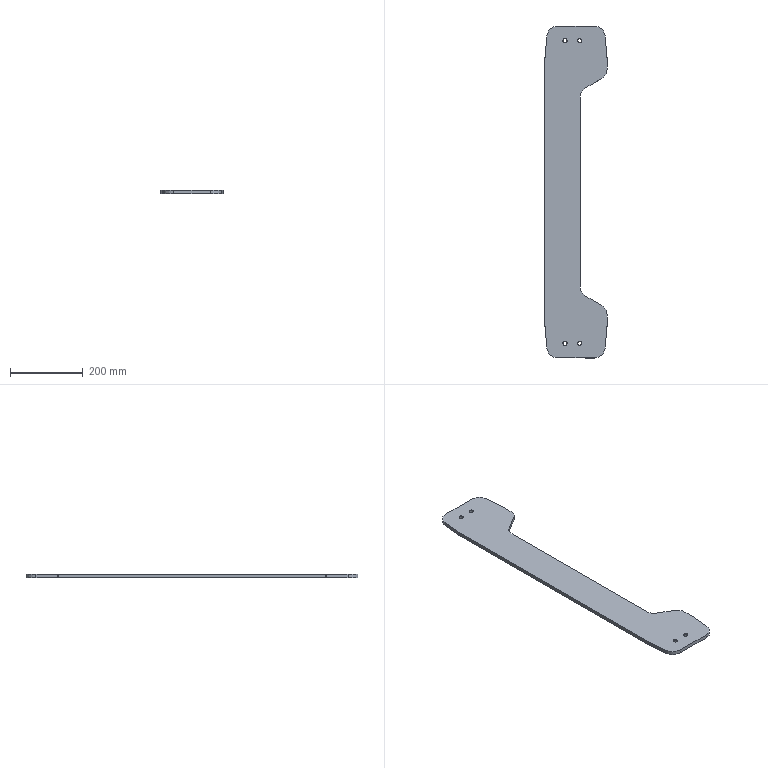Part | SolidWorks | features 3DProfileFeature 1, Extrusion 1, HoleWzd 1 | 1 solid | 42 faces | box 170 x 909.794 x 10 mm | volume 1088199 mm3 | cylinder 20 | plane 14 | cone 8 | commonest cylinder face diameters 60 x12 10.2 x8
STEP:
#1=CARTESIAN_POINT('',(-0.1,-1413.897,9.075));
#2=VERTEX_POINT('',#1);
#3=CARTESIAN_POINT('',(10.1,-1413.897,9.075));
#4=VERTEX_POINT('',#3);
#5=CARTESIAN_POINT('',(5.,-1413.897,9.075));
#6=DIRECTION('',(0.,0.,1.));
#7=DIRECTION('',(1.,0.,0.));
#8=AXIS2_PLACEMENT_3D('',#5,#6,#7);
#9=CIRCLE('',#8,5.1);
#10=EDGE_CURVE('',#2,#4,#9,.T.);
#11=ORIENTED_EDGE('',*,*,#10,.F.);
#12=CARTESIAN_POINT('',(-1.025,-1413.897,10.));
#13=VERTEX_POINT('',#12);
#14=CARTESIAN_POINT('',(-1.025,-1413.897,10.));
#15=DIRECTION('',(-0.7071,0.,0.7071));
#16=VECTOR('',#15,1000.);
#17=LINE('',#14,#16);
#18=EDGE_CURVE('',#2,#13,#17,.T.);
#19=ORIENTED_EDGE('',*,*,#18,.T.);
#20=CARTESIAN_POINT('',(11.025,-1413.897,10.));
#21=VERTEX_POINT('',#20);
#22=CARTESIAN_POINT('',(5.,-1413.897,10.));
#23=DIRECTION('',(0.,0.,1.));
#24=DIRECTION('',(1.,0.,0.));
#25=AXIS2_PLACEMENT_3D('',#22,#23,#24);
#26=CIRCLE('',#25,6.025);
#27=EDGE_CURVE('',#13,#21,#26,.T.);
#28=ORIENTED_EDGE('',*,*,#27,.T.);
#29=CARTESIAN_POINT('',(11.025,-1413.897,10.));
#30=DIRECTION('',(0.7071,0.,0.7071));
#31=VECTOR('',#30,1000.);
#32=LINE('',#29,#31);
#33=EDGE_CURVE('',#4,#21,#32,.T.);
#34=ORIENTED_EDGE('',*,*,#33,.F.);
#35=EDGE_LOOP('',(#11,#19,#28,#34));
#36=FACE_OUTER_BOUND('',#35,.T.);
#37=CARTESIAN_POINT('',(5.,-1413.897,10.));
#38=DIRECTION('',(0.,0.,1.));
#39=DIRECTION('',(1.,0.,0.));
#40=AXIS2_PLACEMENT_3D('',#37,#38,#39);
#41=CONICAL_SURFACE('',#40,6.025,0.7854);
#42=ADVANCED_FACE('',(#36),#41,.F.);
#43=CARTESIAN_POINT('',(-0.1,-1413.897,0.));
#44=VERTEX_POINT('',#43);
#45=CARTESIAN_POINT('',(10.1,-1413.897,0.));
#46=VERTEX_POINT('',#45);
#47=CARTESIAN_POINT('',(5.,-1413.897,0.));
#48=DIRECTION('',(0.,0.,1.));
#49=DIRECTION('',(1.,0.,0.));
#50=AXIS2_PLACEMENT_3D('',#47,#48,#49);
#51=CIRCLE('',#50,5.1);
#52=EDGE_CURVE('',#44,#46,#51,.T.);
#53=ORIENTED_EDGE('',*,*,#52,.F.);
#54=CARTESIAN_POINT('',(-0.1,-1413.897,10.));
#55=DIRECTION('',(0.,0.,1.));
#56=VECTOR('',#55,1000.);
#57=LINE('',#54,#56);
#58=EDGE_CURVE('',#44,#2,#57,.T.);
#59=ORIENTED_EDGE('',*,*,#58,.T.);
#60=ORIENTED_EDGE('',*,*,#10,.T.);
#61=CARTESIAN_POINT('',(10.1,-1413.897,10.));
#62=DIRECTION('',(0.,0.,1.));
#63=VECTOR('',#62,1000.);
#64=LINE('',#61,#63);
#65=EDGE_CURVE('',#46,#4,#64,.T.);
#66=ORIENTED_EDGE('',*,*,#65,.F.);
#67=EDGE_LOOP('',(#53,#59,#60,#66));
#68=FACE_OUTER_BOUND('',#67,.T.);
#69=CARTESIAN_POINT('',(5.,-1413.897,10.));
#70=DIRECTION('',(0.,0.,1.));
#71=DIRECTION('',(1.,0.,0.));
#72=AXIS2_PLACEMENT_3D('',#69,#70,#71);
#73=CYLINDRICAL_SURFACE('',#72,5.1);
#74=ADVANCED_FACE('',(#68),#73,.F.);
#75=CARTESIAN_POINT('',(-40.1,-1413.897,9.075));
#76=VERTEX_POINT('',#75);
#77=CARTESIAN_POINT('',(-29.9,-1413.897,9.075));
#78=VERTEX_POINT('',#77);
#79=CARTESIAN_POINT('',(-35.,-1413.897,9.075));
#80=DIRECTION('',(0.,0.,1.));
#81=DIRECTION('',(1.,0.,0.));
#82=AXIS2_PLACEMENT_3D('',#79,#80,#81);
#83=CIRCLE('',#82,5.1);
#84=EDGE_CURVE('',#76,#78,#83,.T.);
#85=ORIENTED_EDGE('',*,*,#84,.F.);
#86=CARTESIAN_POINT('',(-41.025,-1413.897,10.));
#87=VERTEX_POINT('',#86);
#88=CARTESIAN_POINT('',(-41.025,-1413.897,10.));
#89=DIRECTION('',(-0.7071,0.,0.7071));
#90=VECTOR('',#89,1000.);
#91=LINE('',#88,#90);
#92=EDGE_CURVE('',#76,#87,#91,.T.);
#93=ORIENTED_EDGE('',*,*,#92,.T.);
#94=CARTESIAN_POINT('',(-28.975,-1413.897,10.));
#95=VERTEX_POINT('',#94);
#96=CARTESIAN_POINT('',(-35.,-1413.897,10.));
#97=DIRECTION('',(0.,0.,1.));
#98=DIRECTION('',(1.,0.,0.));
#99=AXIS2_PLACEMENT_3D('',#96,#97,#98);
#100=CIRCLE('',#99,6.025);
#101=EDGE_CURVE('',#87,#95,#100,.T.);
#102=ORIENTED_EDGE('',*,*,#101,.T.);
#103=CARTESIAN_POINT('',(-28.975,-1413.897,10.));
#104=DIRECTION('',(0.7071,0.,0.7071));
#105=VECTOR('',#104,1000.);
#106=LINE('',#103,#105);
#107=EDGE_CURVE('',#78,#95,#106,.T.);
#108=ORIENTED_EDGE('',*,*,#107,.F.);
#109=EDGE_LOOP('',(#85,#93,#102,#108));
#110=FACE_OUTER_BOUND('',#109,.T.);
#111=CARTESIAN_POINT('',(-35.,-1413.897,10.));
#112=DIRECTION('',(0.,0.,1.));
#113=DIRECTION('',(1.,0.,0.));
#114=AXIS2_PLACEMENT_3D('',#111,#112,#113);
#115=CONICAL_SURFACE('',#114,6.025,0.7854);
#116=ADVANCED_FACE('',(#110),#115,.F.);
#117=CARTESIAN_POINT('',(-40.1,-1413.897,0.));
#118=VERTEX_POINT('',#117);
#119=CARTESIAN_POINT('',(-29.9,-1413.897,0.));
#120=VERTEX_POINT('',#119);
#121=CARTESIAN_POINT('',(-35.,-1413.897,0.));
#122=DIRECTION('',(0.,0.,1.));
#123=DIRECTION('',(1.,0.,0.));
#124=AXIS2_PLACEMENT_3D('',#121,#122,#123);
#125=CIRCLE('',#124,5.1);
#126=EDGE_CURVE('',#118,#120,#125,.T.);
#127=ORIENTED_EDGE('',*,*,#126,.F.);
#128=CARTESIAN_POINT('',(-40.1,-1413.897,10.));
#129=DIRECTION('',(0.,0.,1.));
#130=VECTOR('',#129,1000.);
#131=LINE('',#128,#130);
#132=EDGE_CURVE('',#118,#76,#131,.T.);
#133=ORIENTED_EDGE('',*,*,#132,.T.);
#134=ORIENTED_EDGE('',*,*,#84,.T.);
#135=CARTESIAN_POINT('',(-29.9,-1413.897,10.));
#136=DIRECTION('',(0.,0.,1.));
#137=VECTOR('',#136,1000.);
#138=LINE('',#135,#137);
#139=EDGE_CURVE('',#120,#78,#138,.T.);
#140=ORIENTED_EDGE('',*,*,#139,.F.);
#141=EDGE_LOOP('',(#127,#133,#134,#140));
#142=FACE_OUTER_BOUND('',#141,.T.);
#143=CARTESIAN_POINT('',(-35.,-1413.897,10.));
#144=DIRECTION('',(0.,0.,1.));
#145=DIRECTION('',(1.,0.,0.));
#146=AXIS2_PLACEMENT_3D('',#143,#144,#145);
#147=CYLINDRICAL_SURFACE('',#146,5.1);
#148=ADVANCED_FACE('',(#142),#147,.F.);
#149=CARTESIAN_POINT('',(-40.1,-584.103,9.075));
#150=VERTEX_POINT('',#149);
#151=CARTESIAN_POINT('',(-29.9,-584.103,9.075));
#152=VERTEX_POINT('',#151);
#153=CARTESIAN_POINT('',(-35.,-584.103,9.075));
#154=DIRECTION('',(0.,0.,1.));
#155=DIRECTION('',(1.,0.,0.));
#156=AXIS2_PLACEMENT_3D('',#153,#154,#155);
#157=CIRCLE('',#156,5.1);
#158=EDGE_CURVE('',#150,#152,#157,.T.);
#159=ORIENTED_EDGE('',*,*,#158,.F.);
#160=CARTESIAN_POINT('',(-41.025,-584.103,10.));
#161=VERTEX_POINT('',#160);
#162=CARTESIAN_POINT('',(-41.025,-584.103,10.));
#163=DIRECTION('',(-0.7071,0.,0.7071));
#164=VECTOR('',#163,1000.);
#165=LINE('',#162,#164);
#166=EDGE_CURVE('',#150,#161,#165,.T.);
#167=ORIENTED_EDGE('',*,*,#166,.T.);
#168=CARTESIAN_POINT('',(-28.975,-584.103,10.));
#169=VERTEX_POINT('',#168);
#170=CARTESIAN_POINT('',(-35.,-584.103,10.));
#171=DIRECTION('',(0.,0.,1.));
#172=DIRECTION('',(1.,0.,0.));
#173=AXIS2_PLACEMENT_3D('',#170,#171,#172);
#174=CIRCLE('',#173,6.025);
#175=EDGE_CURVE('',#161,#169,#174,.T.);
#176=ORIENTED_EDGE('',*,*,#175,.T.);
#177=CARTESIAN_POINT('',(-28.975,-584.103,10.));
#178=DIRECTION('',(0.7071,0.,0.7071));
#179=VECTOR('',#178,1000.);
#180=LINE('',#177,#179);
#181=EDGE_CURVE('',#152,#169,#180,.T.);
#182=ORIENTED_EDGE('',*,*,#181,.F.);
#183=EDGE_LOOP('',(#159,#167,#176,#182));
#184=FACE_OUTER_BOUND('',#183,.T.);
#185=CARTESIAN_POINT('',(-35.,-584.103,10.));
#186=DIRECTION('',(0.,0.,1.));
#187=DIRECTION('',(1.,0.,0.));
#188=AXIS2_PLACEMENT_3D('',#185,#186,#187);
#189=CONICAL_SURFACE('',#188,6.025,0.7854);
#190=ADVANCED_FACE('',(#184),#189,.F.);
#191=CARTESIAN_POINT('',(-40.1,-584.103,0.));
#192=VERTEX_POINT('',#191);
#193=CARTESIAN_POINT('',(-29.9,-584.103,0.));
#194=VERTEX_POINT('',#193);
#195=CARTESIAN_POINT('',(-35.,-584.103,0.));
#196=DIRECTION('',(0.,0.,1.));
#197=DIRECTION('',(1.,0.,0.));
#198=AXIS2_PLACEMENT_3D('',#195,#196,#197);
#199=CIRCLE('',#198,5.1);
#200=EDGE_CURVE('',#192,#194,#199,.T.);
#201=ORIENTED_EDGE('',*,*,#200,.F.);
#202=CARTESIAN_POINT('',(-40.1,-584.103,10.));
#203=DIRECTION('',(0.,0.,1.));
#204=VECTOR('',#203,1000.);
#205=LINE('',#202,#204);
#206=EDGE_CURVE('',#192,#150,#205,.T.);
#207=ORIENTED_EDGE('',*,*,#206,.T.);
#208=ORIENTED_EDGE('',*,*,#158,.T.);
#209=CARTESIAN_POINT('',(-29.9,-584.103,10.));
#210=DIRECTION('',(0.,0.,1.));
#211=VECTOR('',#210,1000.);
#212=LINE('',#209,#211);
#213=EDGE_CURVE('',#194,#152,#212,.T.);
#214=ORIENTED_EDGE('',*,*,#213,.F.);
#215=EDGE_LOOP('',(#201,#207,#208,#214));
#216=FACE_OUTER_BOUND('',#215,.T.);
#217=CARTESIAN_POINT('',(-35.,-584.103,10.));
#218=DIRECTION('',(0.,0.,1.));
#219=DIRECTION('',(1.,0.,0.));
#220=AXIS2_PLACEMENT_3D('',#217,#218,#219);
#221=CYLINDRICAL_SURFACE('',#220,5.1);
#222=ADVANCED_FACE('',(#216),#221,.F.);
#223=CARTESIAN_POINT('',(-0.1,-584.103,9.075));
#224=VERTEX_POINT('',#223);
#225=CARTESIAN_POINT('',(10.1,-584.103,9.075));
#226=VERTEX_POINT('',#225);
#227=CARTESIAN_POINT('',(5.,-584.103,9.075));
#228=DIRECTION('',(0.,0.,1.));
#229=DIRECTION('',(1.,0.,0.));
#230=AXIS2_PLACEMENT_3D('',#227,#228,#229);
#231=CIRCLE('',#230,5.1);
#232=EDGE_CURVE('',#224,#226,#231,.T.);
#233=ORIENTED_EDGE('',*,*,#232,.F.);
#234=CARTESIAN_POINT('',(-1.025,-584.103,10.));
#235=VERTEX_POINT('',#234);
#236=CARTESIAN_POINT('',(-1.025,-584.103,10.));
#237=DIRECTION('',(-0.7071,0.,0.7071));
#238=VECTOR('',#237,1000.);
#239=LINE('',#236,#238);
#240=EDGE_CURVE('',#224,#235,#239,.T.);
#241=ORIENTED_EDGE('',*,*,#240,.T.);
#242=CARTESIAN_POINT('',(11.025,-584.103,10.));
#243=VERTEX_POINT('',#242);
#244=CARTESIAN_POINT('',(5.,-584.103,10.));
#245=DIRECTION('',(0.,0.,1.));
#246=DIRECTION('',(1.,0.,0.));
#247=AXIS2_PLACEMENT_3D('',#244,#245,#246);
#248=CIRCLE('',#247,6.025);
#249=EDGE_CURVE('',#235,#243,#248,.T.);
#250=ORIENTED_EDGE('',*,*,#249,.T.);
#251=CARTESIAN_POINT('',(11.025,-584.103,10.));
#252=DIRECTION('',(0.7071,0.,0.7071));
#253=VECTOR('',#252,1000.);
#254=LINE('',#251,#253);
#255=EDGE_CURVE('',#226,#243,#254,.T.);
#256=ORIENTED_EDGE('',*,*,#255,.F.);
#257=EDGE_LOOP('',(#233,#241,#250,#256));
#258=FACE_OUTER_BOUND('',#257,.T.);
#259=CARTESIAN_POINT('',(5.,-584.103,10.));
#260=DIRECTION('',(0.,0.,1.));
#261=DIRECTION('',(1.,0.,0.));
#262=AXIS2_PLACEMENT_3D('',#259,#260,#261);
#263=CONICAL_SURFACE('',#262,6.025,0.7854);
#264=ADVANCED_FACE('',(#258),#263,.F.);
#265=CARTESIAN_POINT('',(-0.1,-584.103,0.));
#266=VERTEX_POINT('',#265);
#267=CARTESIAN_POINT('',(10.1,-584.103,0.));
#268=VERTEX_POINT('',#267);
#269=CARTESIAN_POINT('',(5.,-584.103,0.));
#270=DIRECTION('',(0.,0.,1.));
#271=DIRECTION('',(1.,0.,0.));
#272=AXIS2_PLACEMENT_3D('',#269,#270,#271);
#273=CIRCLE('',#272,5.1);
#274=EDGE_CURVE('',#266,#268,#273,.T.);
#275=ORIENTED_EDGE('',*,*,#274,.F.);
#276=CARTESIAN_POINT('',(-0.1,-584.103,10.));
#277=DIRECTION('',(0.,0.,1.));
#278=VECTOR('',#277,1000.);
#279=LINE('',#276,#278);
#280=EDGE_CURVE('',#266,#224,#279,.T.);
#281=ORIENTED_EDGE('',*,*,#280,.T.);
#282=ORIENTED_EDGE('',*,*,#232,.T.);
#283=CARTESIAN_POINT('',(10.1,-584.103,10.));
#284=DIRECTION('',(0.,0.,1.));
#285=VECTOR('',#284,1000.);
#286=LINE('',#283,#285);
#287=EDGE_CURVE('',#268,#226,#286,.T.);
#288=ORIENTED_EDGE('',*,*,#287,.F.);
#289=EDGE_LOOP('',(#275,#281,#282,#288));
#290=FACE_OUTER_BOUND('',#289,.T.);
#291=CARTESIAN_POINT('',(5.,-584.103,10.));
#292=DIRECTION('',(0.,0.,1.));
#293=DIRECTION('',(1.,0.,0.));
#294=AXIS2_PLACEMENT_3D('',#291,#292,#293);
#295=CYLINDRICAL_SURFACE('',#294,5.1);
#296=ADVANCED_FACE('',(#290),#295,.F.);
#297=CARTESIAN_POINT('',(-54.916,-544.103,0.));
#298=VERTEX_POINT('',#297);
#299=CARTESIAN_POINT('',(-84.802,-571.488,0.));
#300=VERTEX_POINT('',#299);
#301=CARTESIAN_POINT('',(-54.916,-574.103,0.));
#302=DIRECTION('',(0.,0.,1.));
#303=DIRECTION('',(1.,0.,0.));
#304=AXIS2_PLACEMENT_3D('',#301,#302,#303);
#305=CIRCLE('',#304,30.);
#306=EDGE_CURVE('',#298,#300,#305,.T.);
#307=ORIENTED_EDGE('',*,*,#306,.T.);
#308=CARTESIAN_POINT('',(-84.802,-571.488,10.));
#309=VERTEX_POINT('',#308);
#310=CARTESIAN_POINT('',(-84.802,-571.488,10.));
#311=DIRECTION('',(0.,0.,-1.));
#312=VECTOR('',#311,1000.);
#313=LINE('',#310,#312);
#314=EDGE_CURVE('',#309,#300,#313,.T.);
#315=ORIENTED_EDGE('',*,*,#314,.F.);
#316=CARTESIAN_POINT('',(-54.916,-544.103,10.));
#317=VERTEX_POINT('',#316);
#318=CARTESIAN_POINT('',(-54.916,-574.103,10.));
#319=DIRECTION('',(0.,0.,1.));
#320=DIRECTION('',(1.,0.,0.));
#321=AXIS2_PLACEMENT_3D('',#318,#319,#320);
#322=CIRCLE('',#321,30.);
#323=EDGE_CURVE('',#317,#309,#322,.T.);
#324=ORIENTED_EDGE('',*,*,#323,.F.);
#325=CARTESIAN_POINT('',(-54.916,-544.103,10.));
#326=DIRECTION('',(0.,0.,-1.));
#327=VECTOR('',#326,1000.);
#328=LINE('',#325,#327);
#329=EDGE_CURVE('',#317,#298,#328,.T.);
#330=ORIENTED_EDGE('',*,*,#329,.T.);
#331=EDGE_LOOP('',(#307,#315,#324,#330));
#332=FACE_OUTER_BOUND('',#331,.T.);
#333=CARTESIAN_POINT('',(-54.916,-574.103,10.));
#334=DIRECTION('',(0.,0.,-1.));
#335=DIRECTION('',(-1.,0.,0.));
#336=AXIS2_PLACEMENT_3D('',#333,#334,#335);
#337=CYLINDRICAL_SURFACE('',#336,30.);
#338=ADVANCED_FACE('',(#332),#337,.T.);
#339=CARTESIAN_POINT('',(-89.886,-629.598,0.));
#340=VERTEX_POINT('',#339);
#341=CARTESIAN_POINT('',(-84.802,-571.488,0.));
#342=DIRECTION('',(-0.08716,-0.9962,0.));
#343=VECTOR('',#342,1000.);
#344=LINE('',#341,#343);
#345=EDGE_CURVE('',#300,#340,#344,.T.);
#346=ORIENTED_EDGE('',*,*,#345,.T.);
#347=CARTESIAN_POINT('',(-89.886,-629.598,10.));
#348=VERTEX_POINT('',#347);
#349=CARTESIAN_POINT('',(-89.886,-629.598,10.));
#350=DIRECTION('',(0.,0.,-1.));
#351=VECTOR('',#350,1000.);
#352=LINE('',#349,#351);
#353=EDGE_CURVE('',#348,#340,#352,.T.);
#354=ORIENTED_EDGE('',*,*,#353,.F.);
#355=CARTESIAN_POINT('',(-84.802,-571.488,10.));
#356=DIRECTION('',(-0.08716,-0.9962,0.));
#357=VECTOR('',#356,1000.);
#358=LINE('',#355,#357);
#359=EDGE_CURVE('',#309,#348,#358,.T.);
#360=ORIENTED_EDGE('',*,*,#359,.F.);
#361=ORIENTED_EDGE('',*,*,#314,.T.);
#362=EDGE_LOOP('',(#346,#354,#360,#361));
#363=FACE_OUTER_BOUND('',#362,.T.);
#364=CARTESIAN_POINT('',(-84.802,-571.488,10.));
#365=DIRECTION('',(0.9962,-0.08716,0.));
#366=DIRECTION('',(0.08716,0.9962,0.));
#367=AXIS2_PLACEMENT_3D('',#364,#365,#366);
#368=PLANE('',#367);
#369=ADVANCED_FACE('',(#363),#368,.F.);
#370=CARTESIAN_POINT('',(-90.,-632.212,0.));
#371=VERTEX_POINT('',#370);
#372=CARTESIAN_POINT('',(-60.,-632.212,0.));
#373=DIRECTION('',(0.,0.,1.));
#374=DIRECTION('',(1.,0.,0.));
#375=AXIS2_PLACEMENT_3D('',#372,#373,#374);
#376=CIRCLE('',#375,30.);
#377=EDGE_CURVE('',#340,#371,#376,.T.);
#378=ORIENTED_EDGE('',*,*,#377,.T.);
#379=CARTESIAN_POINT('',(-90.,-632.212,10.));
#380=VERTEX_POINT('',#379);
#381=CARTESIAN_POINT('',(-90.,-632.212,10.));
#382=DIRECTION('',(0.,0.,-1.));
#383=VECTOR('',#382,1000.);
#384=LINE('',#381,#383);
#385=EDGE_CURVE('',#380,#371,#384,.T.);
#386=ORIENTED_EDGE('',*,*,#385,.F.);
#387=CARTESIAN_POINT('',(-60.,-632.212,10.));
#388=DIRECTION('',(0.,0.,1.));
#389=DIRECTION('',(1.,0.,0.));
#390=AXIS2_PLACEMENT_3D('',#387,#388,#389);
#391=CIRCLE('',#390,30.);
#392=EDGE_CURVE('',#348,#380,#391,.T.);
#393=ORIENTED_EDGE('',*,*,#392,.F.);
#394=ORIENTED_EDGE('',*,*,#353,.T.);
#395=EDGE_LOOP('',(#378,#386,#393,#394));
#396=FACE_OUTER_BOUND('',#395,.T.);
#397=CARTESIAN_POINT('',(-60.,-632.212,10.));
#398=DIRECTION('',(0.,0.,-1.));
#399=DIRECTION('',(-1.,0.,0.));
#400=AXIS2_PLACEMENT_3D('',#397,#398,#399);
#401=CYLINDRICAL_SURFACE('',#400,30.);
#402=ADVANCED_FACE('',(#396),#401,.T.);
#403=CARTESIAN_POINT('',(-90.,-1365.788,0.));
#404=VERTEX_POINT('',#403);
#405=CARTESIAN_POINT('',(-90.,-1365.788,0.));
#406=DIRECTION('',(0.,-1.,0.));
#407=VECTOR('',#406,1000.);
#408=LINE('',#405,#407);
#409=EDGE_CURVE('',#371,#404,#408,.T.);
#410=ORIENTED_EDGE('',*,*,#409,.T.);
#411=CARTESIAN_POINT('',(-90.,-1365.788,10.));
#412=VERTEX_POINT('',#411);
#413=CARTESIAN_POINT('',(-90.,-1365.788,10.));
#414=DIRECTION('',(0.,0.,-1.));
#415=VECTOR('',#414,1000.);
#416=LINE('',#413,#415);
#417=EDGE_CURVE('',#412,#404,#416,.T.);
#418=ORIENTED_EDGE('',*,*,#417,.F.);
#419=CARTESIAN_POINT('',(-90.,-1365.788,10.));
#420=DIRECTION('',(0.,-1.,0.));
#421=VECTOR('',#420,1000.);
#422=LINE('',#419,#421);
#423=EDGE_CURVE('',#380,#412,#422,.T.);
#424=ORIENTED_EDGE('',*,*,#423,.F.);
#425=ORIENTED_EDGE('',*,*,#385,.T.);
#426=EDGE_LOOP('',(#410,#418,#424,#425));
#427=FACE_OUTER_BOUND('',#426,.T.);
#428=CARTESIAN_POINT('',(-90.,-1365.788,10.));
#429=DIRECTION('',(1.,0.,0.));
#430=DIRECTION('',(0.,0.,-1.));
#431=AXIS2_PLACEMENT_3D('',#428,#429,#430);
#432=PLANE('',#431);
#433=ADVANCED_FACE('',(#427),#432,.F.);
#434=CARTESIAN_POINT('',(-89.886,-1368.402,0.));
#435=VERTEX_POINT('',#434);
#436=CARTESIAN_POINT('',(-60.,-1365.788,0.));
#437=DIRECTION('',(0.,0.,1.));
#438=DIRECTION('',(1.,0.,0.));
#439=AXIS2_PLACEMENT_3D('',#436,#437,#438);
#440=CIRCLE('',#439,30.);
#441=EDGE_CURVE('',#404,#435,#440,.T.);
#442=ORIENTED_EDGE('',*,*,#441,.T.);
#443=CARTESIAN_POINT('',(-89.886,-1368.402,10.));
#444=VERTEX_POINT('',#443);
#445=CARTESIAN_POINT('',(-89.886,-1368.402,10.));
#446=DIRECTION('',(0.,0.,-1.));
#447=VECTOR('',#446,1000.);
#448=LINE('',#445,#447);
#449=EDGE_CURVE('',#444,#435,#448,.T.);
#450=ORIENTED_EDGE('',*,*,#449,.F.);
#451=CARTESIAN_POINT('',(-60.,-1365.788,10.));
#452=DIRECTION('',(0.,0.,1.));
#453=DIRECTION('',(1.,0.,0.));
#454=AXIS2_PLACEMENT_3D('',#451,#452,#453);
#455=CIRCLE('',#454,30.);
#456=EDGE_CURVE('',#412,#444,#455,.T.);
#457=ORIENTED_EDGE('',*,*,#456,.F.);
#458=ORIENTED_EDGE('',*,*,#417,.T.);
#459=EDGE_LOOP('',(#442,#450,#457,#458));
#460=FACE_OUTER_BOUND('',#459,.T.);
#461=CARTESIAN_POINT('',(-60.,-1365.788,10.));
#462=DIRECTION('',(0.,0.,-1.));
#463=DIRECTION('',(-1.,0.,0.));
#464=AXIS2_PLACEMENT_3D('',#461,#462,#463);
#465=CYLINDRICAL_SURFACE('',#464,30.);
#466=ADVANCED_FACE('',(#460),#465,.T.);
#467=CARTESIAN_POINT('',(-84.802,-1426.512,0.));
#468=VERTEX_POINT('',#467);
#469=CARTESIAN_POINT('',(-84.802,-1426.512,0.));
#470=DIRECTION('',(0.08716,-0.9962,0.));
#471=VECTOR('',#470,1000.);
#472=LINE('',#469,#471);
#473=EDGE_CURVE('',#435,#468,#472,.T.);
#474=ORIENTED_EDGE('',*,*,#473,.T.);
#475=CARTESIAN_POINT('',(-84.802,-1426.512,10.));
#476=VERTEX_POINT('',#475);
#477=CARTESIAN_POINT('',(-84.802,-1426.512,10.));
#478=DIRECTION('',(0.,0.,-1.));
#479=VECTOR('',#478,1000.);
#480=LINE('',#477,#479);
#481=EDGE_CURVE('',#476,#468,#480,.T.);
#482=ORIENTED_EDGE('',*,*,#481,.F.);
#483=CARTESIAN_POINT('',(-84.802,-1426.512,10.));
#484=DIRECTION('',(0.08716,-0.9962,0.));
#485=VECTOR('',#484,1000.);
#486=LINE('',#483,#485);
#487=EDGE_CURVE('',#444,#476,#486,.T.);
#488=ORIENTED_EDGE('',*,*,#487,.F.);
#489=ORIENTED_EDGE('',*,*,#449,.T.);
#490=EDGE_LOOP('',(#474,#482,#488,#489));
#491=FACE_OUTER_BOUND('',#490,.T.);
#492=CARTESIAN_POINT('',(-84.802,-1426.512,10.));
#493=DIRECTION('',(0.9962,0.08716,0.));
#494=DIRECTION('',(-0.08716,0.9962,0.));
#495=AXIS2_PLACEMENT_3D('',#492,#493,#494);
#496=PLANE('',#495);
#497=ADVANCED_FACE('',(#491),#496,.F.);
#498=CARTESIAN_POINT('',(-54.916,-1453.897,0.));
#499=VERTEX_POINT('',#498);
#500=CARTESIAN_POINT('',(-54.916,-1423.897,0.));
#501=DIRECTION('',(0.,0.,1.));
#502=DIRECTION('',(1.,0.,0.));
#503=AXIS2_PLACEMENT_3D('',#500,#501,#502);
#504=CIRCLE('',#503,30.);
#505=EDGE_CURVE('',#468,#499,#504,.T.);
#506=ORIENTED_EDGE('',*,*,#505,.T.);
#507=CARTESIAN_POINT('',(-54.916,-1453.897,10.));
#508=VERTEX_POINT('',#507);
#509=CARTESIAN_POINT('',(-54.916,-1453.897,10.));
#510=DIRECTION('',(0.,0.,-1.));
#511=VECTOR('',#510,1000.);
#512=LINE('',#509,#511);
#513=EDGE_CURVE('',#508,#499,#512,.T.);
#514=ORIENTED_EDGE('',*,*,#513,.F.);
#515=CARTESIAN_POINT('',(-54.916,-1423.897,10.));
#516=DIRECTION('',(0.,0.,1.));
#517=DIRECTION('',(1.,0.,0.));
#518=AXIS2_PLACEMENT_3D('',#515,#516,#517);
#519=CIRCLE('',#518,30.);
#520=EDGE_CURVE('',#476,#508,#519,.T.);
#521=ORIENTED_EDGE('',*,*,#520,.F.);
#522=ORIENTED_EDGE('',*,*,#481,.T.);
#523=EDGE_LOOP('',(#506,#514,#521,#522));
#524=FACE_OUTER_BOUND('',#523,.T.);
#525=CARTESIAN_POINT('',(-54.916,-1423.897,10.));
#526=DIRECTION('',(0.,0.,-1.));
#527=DIRECTION('',(-1.,0.,0.));
#528=AXIS2_PLACEMENT_3D('',#525,#526,#527);
#529=CYLINDRICAL_SURFACE('',#528,30.);
#530=ADVANCED_FACE('',(#524),#529,.T.);
#531=CARTESIAN_POINT('',(44.916,-1453.897,0.));
#532=VERTEX_POINT('',#531);
#533=CARTESIAN_POINT('',(-54.916,-1453.897,0.));
#534=DIRECTION('',(1.,0.,0.));
#535=VECTOR('',#534,1000.);
#536=LINE('',#533,#535);
#537=EDGE_CURVE('',#499,#532,#536,.T.);
#538=ORIENTED_EDGE('',*,*,#537,.T.);
#539=CARTESIAN_POINT('',(44.916,-1453.897,10.));
#540=VERTEX_POINT('',#539);
#541=CARTESIAN_POINT('',(44.916,-1453.897,10.));
#542=DIRECTION('',(0.,0.,-1.));
#543=VECTOR('',#542,1000.);
#544=LINE('',#541,#543);
#545=EDGE_CURVE('',#540,#532,#544,.T.);
#546=ORIENTED_EDGE('',*,*,#545,.F.);
#547=CARTESIAN_POINT('',(-54.916,-1453.897,10.));
#548=DIRECTION('',(1.,0.,0.));
#549=VECTOR('',#548,1000.);
#550=LINE('',#547,#549);
#551=EDGE_CURVE('',#508,#540,#550,.T.);
#552=ORIENTED_EDGE('',*,*,#551,.F.);
#553=ORIENTED_EDGE('',*,*,#513,.T.);
#554=EDGE_LOOP('',(#538,#546,#552,#553));
#555=FACE_OUTER_BOUND('',#554,.T.);
#556=CARTESIAN_POINT('',(-54.916,-1453.897,10.));
#557=DIRECTION('',(0.,1.,0.));
#558=DIRECTION('',(0.,0.,1.));
#559=AXIS2_PLACEMENT_3D('',#556,#557,#558);
#560=PLANE('',#559);
#561=ADVANCED_FACE('',(#555),#560,.F.);
#562=CARTESIAN_POINT('',(74.802,-1426.512,0.));
#563=VERTEX_POINT('',#562);
#564=CARTESIAN_POINT('',(44.916,-1423.897,0.));
#565=DIRECTION('',(0.,0.,1.));
#566=DIRECTION('',(-1.,0.,0.));
#567=AXIS2_PLACEMENT_3D('',#564,#565,#566);
#568=CIRCLE('',#567,30.);
#569=EDGE_CURVE('',#532,#563,#568,.T.);
#570=ORIENTED_EDGE('',*,*,#569,.T.);
#571=CARTESIAN_POINT('',(74.802,-1426.512,10.));
#572=VERTEX_POINT('',#571);
#573=CARTESIAN_POINT('',(74.802,-1426.512,10.));
#574=DIRECTION('',(0.,0.,-1.));
#575=VECTOR('',#574,1000.);
#576=LINE('',#573,#575);
#577=EDGE_CURVE('',#572,#563,#576,.T.);
#578=ORIENTED_EDGE('',*,*,#577,.F.);
#579=CARTESIAN_POINT('',(44.916,-1423.897,10.));
#580=DIRECTION('',(0.,0.,1.));
#581=DIRECTION('',(-1.,0.,0.));
#582=AXIS2_PLACEMENT_3D('',#579,#580,#581);
#583=CIRCLE('',#582,30.);
#584=EDGE_CURVE('',#540,#572,#583,.T.);
#585=ORIENTED_EDGE('',*,*,#584,.F.);
#586=ORIENTED_EDGE('',*,*,#545,.T.);
#587=EDGE_LOOP('',(#570,#578,#585,#586));
#588=FACE_OUTER_BOUND('',#587,.T.);
#589=CARTESIAN_POINT('',(44.916,-1423.897,10.));
#590=DIRECTION('',(0.,0.,-1.));
#591=DIRECTION('',(-1.,0.,0.));
#592=AXIS2_PLACEMENT_3D('',#589,#590,#591);
#593=CYLINDRICAL_SURFACE('',#592,30.);
#594=ADVANCED_FACE('',(#588),#593,.T.);
#595=CARTESIAN_POINT('',(79.886,-1368.402,0.));
#596=VERTEX_POINT('',#595);
#597=CARTESIAN_POINT('',(74.802,-1426.512,0.));
#598=DIRECTION('',(0.08716,0.9962,0.));
#599=VECTOR('',#598,1000.);
#600=LINE('',#597,#599);
#601=EDGE_CURVE('',#563,#596,#600,.T.);
#602=ORIENTED_EDGE('',*,*,#601,.T.);
#603=CARTESIAN_POINT('',(79.886,-1368.402,10.));
#604=VERTEX_POINT('',#603);
#605=CARTESIAN_POINT('',(79.886,-1368.402,10.));
#606=DIRECTION('',(0.,0.,-1.));
#607=VECTOR('',#606,1000.);
#608=LINE('',#605,#607);
#609=EDGE_CURVE('',#604,#596,#608,.T.);
#610=ORIENTED_EDGE('',*,*,#609,.F.);
#611=CARTESIAN_POINT('',(74.802,-1426.512,10.));
#612=DIRECTION('',(0.08716,0.9962,0.));
#613=VECTOR('',#612,1000.);
#614=LINE('',#611,#613);
#615=EDGE_CURVE('',#572,#604,#614,.T.);
#616=ORIENTED_EDGE('',*,*,#615,.F.);
#617=ORIENTED_EDGE('',*,*,#577,.T.);
#618=EDGE_LOOP('',(#602,#610,#616,#617));
#619=FACE_OUTER_BOUND('',#618,.T.);
#620=CARTESIAN_POINT('',(74.802,-1426.512,10.));
#621=DIRECTION('',(-0.9962,0.08716,0.));
#622=DIRECTION('',(-0.08716,-0.9962,0.));
#623=AXIS2_PLACEMENT_3D('',#620,#621,#622);
#624=PLANE('',#623);
#625=ADVANCED_FACE('',(#619),#624,.F.);
#626=CARTESIAN_POINT('',(80.,-1365.788,0.));
#627=VERTEX_POINT('',#626);
#628=CARTESIAN_POINT('',(50.,-1365.788,0.));
#629=DIRECTION('',(0.,0.,1.));
#630=DIRECTION('',(-1.,0.,0.));
#631=AXIS2_PLACEMENT_3D('',#628,#629,#630);
#632=CIRCLE('',#631,30.);
#633=EDGE_CURVE('',#596,#627,#632,.T.);
#634=ORIENTED_EDGE('',*,*,#633,.T.);
#635=CARTESIAN_POINT('',(80.,-1365.788,10.));
#636=VERTEX_POINT('',#635);
#637=CARTESIAN_POINT('',(80.,-1365.788,10.));
#638=DIRECTION('',(0.,0.,-1.));
#639=VECTOR('',#638,1000.);
#640=LINE('',#637,#639);
#641=EDGE_CURVE('',#636,#627,#640,.T.);
#642=ORIENTED_EDGE('',*,*,#641,.F.);
#643=CARTESIAN_POINT('',(50.,-1365.788,10.));
#644=DIRECTION('',(0.,0.,1.));
#645=DIRECTION('',(-1.,0.,0.));
#646=AXIS2_PLACEMENT_3D('',#643,#644,#645);
#647=CIRCLE('',#646,30.);
#648=EDGE_CURVE('',#604,#636,#647,.T.);
#649=ORIENTED_EDGE('',*,*,#648,.F.);
#650=ORIENTED_EDGE('',*,*,#609,.T.);
#651=EDGE_LOOP('',(#634,#642,#649,#650));
#652=FACE_OUTER_BOUND('',#651,.T.);
#653=CARTESIAN_POINT('',(50.,-1365.788,10.));
#654=DIRECTION('',(0.,0.,-1.));
#655=DIRECTION('',(-1.,0.,0.));
#656=AXIS2_PLACEMENT_3D('',#653,#654,#655);
#657=CYLINDRICAL_SURFACE('',#656,30.);
#658=ADVANCED_FACE('',(#652),#657,.T.);
#659=CARTESIAN_POINT('',(80.,-1335.788,0.));
#660=VERTEX_POINT('',#659);
#661=CARTESIAN_POINT('',(80.,-1365.788,0.));
#662=DIRECTION('',(0.,1.,0.));
#663=VECTOR('',#662,1000.);
#664=LINE('',#661,#663);
#665=EDGE_CURVE('',#627,#660,#664,.T.);
#666=ORIENTED_EDGE('',*,*,#665,.T.);
#667=CARTESIAN_POINT('',(80.,-1335.788,10.));
#668=VERTEX_POINT('',#667);
#669=CARTESIAN_POINT('',(80.,-1335.788,10.));
#670=DIRECTION('',(0.,0.,-1.));
#671=VECTOR('',#670,1000.);
#672=LINE('',#669,#671);
#673=EDGE_CURVE('',#668,#660,#672,.T.);
#674=ORIENTED_EDGE('',*,*,#673,.F.);
#675=CARTESIAN_POINT('',(80.,-1365.788,10.));
#676=DIRECTION('',(0.,1.,0.));
#677=VECTOR('',#676,1000.);
#678=LINE('',#675,#677);
#679=EDGE_CURVE('',#636,#668,#678,.T.);
#680=ORIENTED_EDGE('',*,*,#679,.F.);
#681=ORIENTED_EDGE('',*,*,#641,.T.);
#682=EDGE_LOOP('',(#666,#674,#680,#681));
#683=FACE_OUTER_BOUND('',#682,.T.);
#684=CARTESIAN_POINT('',(80.,-1365.788,10.));
#685=DIRECTION('',(-1.,0.,0.));
#686=DIRECTION('',(0.,0.,1.));
#687=AXIS2_PLACEMENT_3D('',#684,#685,#686);
#688=PLANE('',#687);
#689=ADVANCED_FACE('',(#683),#688,.F.);
#690=CARTESIAN_POINT('',(65.,-1309.807,0.));
#691=VERTEX_POINT('',#690);
#692=CARTESIAN_POINT('',(50.,-1335.788,0.));
#693=DIRECTION('',(0.,0.,1.));
#694=DIRECTION('',(-1.,0.,0.));
#695=AXIS2_PLACEMENT_3D('',#692,#693,#694);
#696=CIRCLE('',#695,30.);
#697=EDGE_CURVE('',#660,#691,#696,.T.);
#698=ORIENTED_EDGE('',*,*,#697,.T.);
#699=CARTESIAN_POINT('',(65.,-1309.807,10.));
#700=VERTEX_POINT('',#699);
#701=CARTESIAN_POINT('',(65.,-1309.807,10.));
#702=DIRECTION('',(0.,0.,-1.));
#703=VECTOR('',#702,1000.);
#704=LINE('',#701,#703);
#705=EDGE_CURVE('',#700,#691,#704,.T.);
#706=ORIENTED_EDGE('',*,*,#705,.F.);
#707=CARTESIAN_POINT('',(50.,-1335.788,10.));
#708=DIRECTION('',(0.,0.,1.));
#709=DIRECTION('',(-1.,0.,0.));
#710=AXIS2_PLACEMENT_3D('',#707,#708,#709);
#711=CIRCLE('',#710,30.);
#712=EDGE_CURVE('',#668,#700,#711,.T.);
#713=ORIENTED_EDGE('',*,*,#712,.F.);
#714=ORIENTED_EDGE('',*,*,#673,.T.);
#715=EDGE_LOOP('',(#698,#706,#713,#714));
#716=FACE_OUTER_BOUND('',#715,.T.);
#717=CARTESIAN_POINT('',(50.,-1335.788,10.));
#718=DIRECTION('',(0.,0.,-1.));
#719=DIRECTION('',(-1.,0.,0.));
#720=AXIS2_PLACEMENT_3D('',#717,#718,#719);
#721=CYLINDRICAL_SURFACE('',#720,30.);
#722=ADVANCED_FACE('',(#716),#721,.T.);
#723=CARTESIAN_POINT('',(22.,-1284.981,0.));
#724=VERTEX_POINT('',#723);
#725=CARTESIAN_POINT('',(65.,-1309.807,0.));
#726=DIRECTION('',(-0.866,0.5,0.));
#727=VECTOR('',#726,1000.);
#728=LINE('',#725,#727);
#729=EDGE_CURVE('',#691,#724,#728,.T.);
#730=ORIENTED_EDGE('',*,*,#729,.T.);
#731=CARTESIAN_POINT('',(22.,-1284.981,10.));
#732=VERTEX_POINT('',#731);
#733=CARTESIAN_POINT('',(22.,-1284.981,10.));
#734=DIRECTION('',(0.,0.,-1.));
#735=VECTOR('',#734,1000.);
#736=LINE('',#733,#735);
#737=EDGE_CURVE('',#732,#724,#736,.T.);
#738=ORIENTED_EDGE('',*,*,#737,.F.);
#739=CARTESIAN_POINT('',(65.,-1309.807,10.));
#740=DIRECTION('',(-0.866,0.5,0.));
#741=VECTOR('',#740,1000.);
#742=LINE('',#739,#741);
#743=EDGE_CURVE('',#700,#732,#742,.T.);
#744=ORIENTED_EDGE('',*,*,#743,.F.);
#745=ORIENTED_EDGE('',*,*,#705,.T.);
#746=EDGE_LOOP('',(#730,#738,#744,#745));
#747=FACE_OUTER_BOUND('',#746,.T.);
#748=CARTESIAN_POINT('',(65.,-1309.807,10.));
#749=DIRECTION('',(-0.5,-0.866,0.));
#750=DIRECTION('',(0.866,-0.5,0.));
#751=AXIS2_PLACEMENT_3D('',#748,#749,#750);
#752=PLANE('',#751);
#753=ADVANCED_FACE('',(#747),#752,.F.);
#754=CARTESIAN_POINT('',(7.,-1259.,0.));
#755=VERTEX_POINT('',#754);
#756=CARTESIAN_POINT('',(37.,-1259.,0.));
#757=DIRECTION('',(0.,0.,-1.));
#758=DIRECTION('',(-1.,0.,0.));
#759=AXIS2_PLACEMENT_3D('',#756,#757,#758);
#760=CIRCLE('',#759,30.);
#761=EDGE_CURVE('',#724,#755,#760,.T.);
#762=ORIENTED_EDGE('',*,*,#761,.T.);
#763=CARTESIAN_POINT('',(7.,-1259.,10.));
#764=VERTEX_POINT('',#763);
#765=CARTESIAN_POINT('',(7.,-1259.,10.));
#766=DIRECTION('',(0.,0.,-1.));
#767=VECTOR('',#766,1000.);
#768=LINE('',#765,#767);
#769=EDGE_CURVE('',#764,#755,#768,.T.);
#770=ORIENTED_EDGE('',*,*,#769,.F.);
#771=CARTESIAN_POINT('',(37.,-1259.,10.));
#772=DIRECTION('',(0.,0.,-1.));
#773=DIRECTION('',(-1.,0.,0.));
#774=AXIS2_PLACEMENT_3D('',#771,#772,#773);
#775=CIRCLE('',#774,30.);
#776=EDGE_CURVE('',#732,#764,#775,.T.);
#777=ORIENTED_EDGE('',*,*,#776,.F.);
#778=ORIENTED_EDGE('',*,*,#737,.T.);
#779=EDGE_LOOP('',(#762,#770,#777,#778));
#780=FACE_OUTER_BOUND('',#779,.T.);
#781=CARTESIAN_POINT('',(37.,-1259.,10.));
#782=DIRECTION('',(0.,0.,-1.));
#783=DIRECTION('',(-1.,0.,0.));
#784=AXIS2_PLACEMENT_3D('',#781,#782,#783);
#785=CYLINDRICAL_SURFACE('',#784,30.);
#786=ADVANCED_FACE('',(#780),#785,.F.);
#787=CARTESIAN_POINT('',(7.,-739.,0.));
#788=VERTEX_POINT('',#787);
#789=CARTESIAN_POINT('',(7.,-1259.,0.));
#790=DIRECTION('',(0.,1.,0.));
#791=VECTOR('',#790,1000.);
#792=LINE('',#789,#791);
#793=EDGE_CURVE('',#755,#788,#792,.T.);
#794=ORIENTED_EDGE('',*,*,#793,.T.);
#795=CARTESIAN_POINT('',(7.,-739.,10.));
#796=VERTEX_POINT('',#795);
#797=CARTESIAN_POINT('',(7.,-739.,10.));
#798=DIRECTION('',(0.,0.,-1.));
#799=VECTOR('',#798,1000.);
#800=LINE('',#797,#799);
#801=EDGE_CURVE('',#796,#788,#800,.T.);
#802=ORIENTED_EDGE('',*,*,#801,.F.);
#803=CARTESIAN_POINT('',(7.,-1259.,10.));
#804=DIRECTION('',(0.,1.,0.));
#805=VECTOR('',#804,1000.);
#806=LINE('',#803,#805);
#807=EDGE_CURVE('',#764,#796,#806,.T.);
#808=ORIENTED_EDGE('',*,*,#807,.F.);
#809=ORIENTED_EDGE('',*,*,#769,.T.);
#810=EDGE_LOOP('',(#794,#802,#808,#809));
#811=FACE_OUTER_BOUND('',#810,.T.);
#812=CARTESIAN_POINT('',(7.,-1259.,10.));
#813=DIRECTION('',(-1.,0.,0.));
#814=DIRECTION('',(0.,-1.,0.));
#815=AXIS2_PLACEMENT_3D('',#812,#813,#814);
#816=PLANE('',#815);
#817=ADVANCED_FACE('',(#811),#816,.F.);
#818=CARTESIAN_POINT('',(22.,-713.019,0.));
#819=VERTEX_POINT('',#818);
#820=CARTESIAN_POINT('',(37.,-739.,0.));
#821=DIRECTION('',(0.,0.,-1.));
#822=DIRECTION('',(1.,0.,0.));
#823=AXIS2_PLACEMENT_3D('',#820,#821,#822);
#824=CIRCLE('',#823,30.);
#825=EDGE_CURVE('',#788,#819,#824,.T.);
#826=ORIENTED_EDGE('',*,*,#825,.T.);
#827=CARTESIAN_POINT('',(22.,-713.019,10.));
#828=VERTEX_POINT('',#827);
#829=CARTESIAN_POINT('',(22.,-713.019,10.));
#830=DIRECTION('',(0.,0.,-1.));
#831=VECTOR('',#830,1000.);
#832=LINE('',#829,#831);
#833=EDGE_CURVE('',#828,#819,#832,.T.);
#834=ORIENTED_EDGE('',*,*,#833,.F.);
#835=CARTESIAN_POINT('',(37.,-739.,10.));
#836=DIRECTION('',(0.,0.,-1.));
#837=DIRECTION('',(1.,0.,0.));
#838=AXIS2_PLACEMENT_3D('',#835,#836,#837);
#839=CIRCLE('',#838,30.);
#840=EDGE_CURVE('',#796,#828,#839,.T.);
#841=ORIENTED_EDGE('',*,*,#840,.F.);
#842=ORIENTED_EDGE('',*,*,#801,.T.);
#843=EDGE_LOOP('',(#826,#834,#841,#842));
#844=FACE_OUTER_BOUND('',#843,.T.);
#845=CARTESIAN_POINT('',(37.,-739.,10.));
#846=DIRECTION('',(0.,0.,-1.));
#847=DIRECTION('',(-1.,0.,0.));
#848=AXIS2_PLACEMENT_3D('',#845,#846,#847);
#849=CYLINDRICAL_SURFACE('',#848,30.);
#850=ADVANCED_FACE('',(#844),#849,.F.);
#851=CARTESIAN_POINT('',(65.,-688.193,0.));
#852=VERTEX_POINT('',#851);
#853=CARTESIAN_POINT('',(65.,-688.193,0.));
#854=DIRECTION('',(0.866,0.5,0.));
#855=VECTOR('',#854,1000.);
#856=LINE('',#853,#855);
#857=EDGE_CURVE('',#819,#852,#856,.T.);
#858=ORIENTED_EDGE('',*,*,#857,.T.);
#859=CARTESIAN_POINT('',(65.,-688.193,10.));
#860=VERTEX_POINT('',#859);
#861=CARTESIAN_POINT('',(65.,-688.193,10.));
#862=DIRECTION('',(0.,0.,-1.));
#863=VECTOR('',#862,1000.);
#864=LINE('',#861,#863);
#865=EDGE_CURVE('',#860,#852,#864,.T.);
#866=ORIENTED_EDGE('',*,*,#865,.F.);
#867=CARTESIAN_POINT('',(65.,-688.193,10.));
#868=DIRECTION('',(0.866,0.5,0.));
#869=VECTOR('',#868,1000.);
#870=LINE('',#867,#869);
#871=EDGE_CURVE('',#828,#860,#870,.T.);
#872=ORIENTED_EDGE('',*,*,#871,.F.);
#873=ORIENTED_EDGE('',*,*,#833,.T.);
#874=EDGE_LOOP('',(#858,#866,#872,#873));
#875=FACE_OUTER_BOUND('',#874,.T.);
#876=CARTESIAN_POINT('',(65.,-688.193,10.));
#877=DIRECTION('',(-0.5,0.866,0.));
#878=DIRECTION('',(-0.866,-0.5,0.));
#879=AXIS2_PLACEMENT_3D('',#876,#877,#878);
#880=PLANE('',#879);
#881=ADVANCED_FACE('',(#875),#880,.F.);
#882=CARTESIAN_POINT('',(80.,-662.212,0.));
#883=VERTEX_POINT('',#882);
#884=CARTESIAN_POINT('',(50.,-662.212,0.));
#885=DIRECTION('',(0.,0.,1.));
#886=DIRECTION('',(-1.,0.,0.));
#887=AXIS2_PLACEMENT_3D('',#884,#885,#886);
#888=CIRCLE('',#887,30.);
#889=EDGE_CURVE('',#852,#883,#888,.T.);
#890=ORIENTED_EDGE('',*,*,#889,.T.);
#891=CARTESIAN_POINT('',(80.,-662.212,10.));
#892=VERTEX_POINT('',#891);
#893=CARTESIAN_POINT('',(80.,-662.212,10.));
#894=DIRECTION('',(0.,0.,-1.));
#895=VECTOR('',#894,1000.);
#896=LINE('',#893,#895);
#897=EDGE_CURVE('',#892,#883,#896,.T.);
#898=ORIENTED_EDGE('',*,*,#897,.F.);
#899=CARTESIAN_POINT('',(50.,-662.212,10.));
#900=DIRECTION('',(0.,0.,1.));
#901=DIRECTION('',(-1.,0.,0.));
#902=AXIS2_PLACEMENT_3D('',#899,#900,#901);
#903=CIRCLE('',#902,30.);
#904=EDGE_CURVE('',#860,#892,#903,.T.);
#905=ORIENTED_EDGE('',*,*,#904,.F.);
#906=ORIENTED_EDGE('',*,*,#865,.T.);
#907=EDGE_LOOP('',(#890,#898,#905,#906));
#908=FACE_OUTER_BOUND('',#907,.T.);
#909=CARTESIAN_POINT('',(50.,-662.212,10.));
#910=DIRECTION('',(0.,0.,-1.));
#911=DIRECTION('',(-1.,0.,0.));
#912=AXIS2_PLACEMENT_3D('',#909,#910,#911);
#913=CYLINDRICAL_SURFACE('',#912,30.);
#914=ADVANCED_FACE('',(#908),#913,.T.);
#915=CARTESIAN_POINT('',(80.,-632.212,0.));
#916=VERTEX_POINT('',#915);
#917=CARTESIAN_POINT('',(80.,-632.212,0.));
#918=DIRECTION('',(0.,1.,0.));
#919=VECTOR('',#918,1000.);
#920=LINE('',#917,#919);
#921=EDGE_CURVE('',#883,#916,#920,.T.);
#922=ORIENTED_EDGE('',*,*,#921,.T.);
#923=CARTESIAN_POINT('',(80.,-632.212,10.));
#924=VERTEX_POINT('',#923);
#925=CARTESIAN_POINT('',(80.,-632.212,10.));
#926=DIRECTION('',(0.,0.,-1.));
#927=VECTOR('',#926,1000.);
#928=LINE('',#925,#927);
#929=EDGE_CURVE('',#924,#916,#928,.T.);
#930=ORIENTED_EDGE('',*,*,#929,.F.);
#931=CARTESIAN_POINT('',(80.,-632.212,10.));
#932=DIRECTION('',(0.,1.,0.));
#933=VECTOR('',#932,1000.);
#934=LINE('',#931,#933);
#935=EDGE_CURVE('',#892,#924,#934,.T.);
#936=ORIENTED_EDGE('',*,*,#935,.F.);
#937=ORIENTED_EDGE('',*,*,#897,.T.);
#938=EDGE_LOOP('',(#922,#930,#936,#937));
#939=FACE_OUTER_BOUND('',#938,.T.);
#940=CARTESIAN_POINT('',(80.,-632.212,10.));
#941=DIRECTION('',(-1.,0.,0.));
#942=DIRECTION('',(0.,0.,1.));
#943=AXIS2_PLACEMENT_3D('',#940,#941,#942);
#944=PLANE('',#943);
#945=ADVANCED_FACE('',(#939),#944,.F.);
#946=CARTESIAN_POINT('',(79.886,-629.598,0.));
#947=VERTEX_POINT('',#946);
#948=CARTESIAN_POINT('',(50.,-632.212,0.));
#949=DIRECTION('',(0.,0.,1.));
#950=DIRECTION('',(-1.,0.,0.));
#951=AXIS2_PLACEMENT_3D('',#948,#949,#950);
#952=CIRCLE('',#951,30.);
#953=EDGE_CURVE('',#916,#947,#952,.T.);
#954=ORIENTED_EDGE('',*,*,#953,.T.);
#955=CARTESIAN_POINT('',(79.886,-629.598,10.));
#956=VERTEX_POINT('',#955);
#957=CARTESIAN_POINT('',(79.886,-629.598,10.));
#958=DIRECTION('',(0.,0.,-1.));
#959=VECTOR('',#958,1000.);
#960=LINE('',#957,#959);
#961=EDGE_CURVE('',#956,#947,#960,.T.);
#962=ORIENTED_EDGE('',*,*,#961,.F.);
#963=CARTESIAN_POINT('',(50.,-632.212,10.));
#964=DIRECTION('',(0.,0.,1.));
#965=DIRECTION('',(-1.,0.,0.));
#966=AXIS2_PLACEMENT_3D('',#963,#964,#965);
#967=CIRCLE('',#966,30.);
#968=EDGE_CURVE('',#924,#956,#967,.T.);
#969=ORIENTED_EDGE('',*,*,#968,.F.);
#970=ORIENTED_EDGE('',*,*,#929,.T.);
#971=EDGE_LOOP('',(#954,#962,#969,#970));
#972=FACE_OUTER_BOUND('',#971,.T.);
#973=CARTESIAN_POINT('',(50.,-632.212,10.));
#974=DIRECTION('',(0.,0.,-1.));
#975=DIRECTION('',(-1.,0.,0.));
#976=AXIS2_PLACEMENT_3D('',#973,#974,#975);
#977=CYLINDRICAL_SURFACE('',#976,30.);
#978=ADVANCED_FACE('',(#972),#977,.T.);
#979=CARTESIAN_POINT('',(74.802,-571.488,0.));
#980=VERTEX_POINT('',#979);
#981=CARTESIAN_POINT('',(74.802,-571.488,0.));
#982=DIRECTION('',(-0.08716,0.9962,0.));
#983=VECTOR('',#982,1000.);
#984=LINE('',#981,#983);
#985=EDGE_CURVE('',#947,#980,#984,.T.);
#986=ORIENTED_EDGE('',*,*,#985,.T.);
#987=CARTESIAN_POINT('',(74.802,-571.488,10.));
#988=VERTEX_POINT('',#987);
#989=CARTESIAN_POINT('',(74.802,-571.488,10.));
#990=DIRECTION('',(0.,0.,-1.));
#991=VECTOR('',#990,1000.);
#992=LINE('',#989,#991);
#993=EDGE_CURVE('',#988,#980,#992,.T.);
#994=ORIENTED_EDGE('',*,*,#993,.F.);
#995=CARTESIAN_POINT('',(74.802,-571.488,10.));
#996=DIRECTION('',(-0.08716,0.9962,0.));
#997=VECTOR('',#996,1000.);
#998=LINE('',#995,#997);
#999=EDGE_CURVE('',#956,#988,#998,.T.);
#1000=ORIENTED_EDGE('',*,*,#999,.F.);
#1001=ORIENTED_EDGE('',*,*,#961,.T.);
#1002=EDGE_LOOP('',(#986,#994,#1000,#1001));
#1003=FACE_OUTER_BOUND('',#1002,.T.);
#1004=CARTESIAN_POINT('',(74.802,-571.488,10.));
#1005=DIRECTION('',(-0.9962,-0.08716,0.));
#1006=DIRECTION('',(0.08716,-0.9962,0.));
#1007=AXIS2_PLACEMENT_3D('',#1004,#1005,#1006);
#1008=PLANE('',#1007);
#1009=ADVANCED_FACE('',(#1003),#1008,.F.);
#1010=CARTESIAN_POINT('',(44.916,-544.103,0.));
#1011=VERTEX_POINT('',#1010);
#1012=CARTESIAN_POINT('',(44.916,-574.103,0.));
#1013=DIRECTION('',(0.,0.,1.));
#1014=DIRECTION('',(1.,0.,0.));
#1015=AXIS2_PLACEMENT_3D('',#1012,#1013,#1014);
#1016=CIRCLE('',#1015,30.);
#1017=EDGE_CURVE('',#980,#1011,#1016,.T.);
#1018=ORIENTED_EDGE('',*,*,#1017,.T.);
#1019=CARTESIAN_POINT('',(44.916,-544.103,10.));
#1020=VERTEX_POINT('',#1019);
#1021=CARTESIAN_POINT('',(44.916,-544.103,10.));
#1022=DIRECTION('',(0.,0.,-1.));
#1023=VECTOR('',#1022,1000.);
#1024=LINE('',#1021,#1023);
#1025=EDGE_CURVE('',#1020,#1011,#1024,.T.);
#1026=ORIENTED_EDGE('',*,*,#1025,.F.);
#1027=CARTESIAN_POINT('',(44.916,-574.103,10.));
#1028=DIRECTION('',(0.,0.,1.));
#1029=DIRECTION('',(1.,0.,0.));
#1030=AXIS2_PLACEMENT_3D('',#1027,#1028,#1029);
#1031=CIRCLE('',#1030,30.);
#1032=EDGE_CURVE('',#988,#1020,#1031,.T.);
#1033=ORIENTED_EDGE('',*,*,#1032,.F.);
#1034=ORIENTED_EDGE('',*,*,#993,.T.);
#1035=EDGE_LOOP('',(#1018,#1026,#1033,#1034));
#1036=FACE_OUTER_BOUND('',#1035,.T.);
#1037=CARTESIAN_POINT('',(44.916,-574.103,10.));
#1038=DIRECTION('',(0.,0.,-1.));
#1039=DIRECTION('',(-1.,0.,0.));
#1040=AXIS2_PLACEMENT_3D('',#1037,#1038,#1039);
#1041=CYLINDRICAL_SURFACE('',#1040,30.);
#1042=ADVANCED_FACE('',(#1036),#1041,.T.);
#1043=CARTESIAN_POINT('',(-54.916,-544.103,0.));
#1044=DIRECTION('',(-1.,0.,0.));
#1045=VECTOR('',#1044,1000.);
#1046=LINE('',#1043,#1045);
#1047=EDGE_CURVE('',#1011,#298,#1046,.T.);
#1048=ORIENTED_EDGE('',*,*,#1047,.T.);
#1049=ORIENTED_EDGE('',*,*,#329,.F.);
#1050=CARTESIAN_POINT('',(-54.916,-544.103,10.));
#1051=DIRECTION('',(-1.,0.,0.));
#1052=VECTOR('',#1051,1000.);
#1053=LINE('',#1050,#1052);
#1054=EDGE_CURVE('',#1020,#317,#1053,.T.);
#1055=ORIENTED_EDGE('',*,*,#1054,.F.);
#1056=ORIENTED_EDGE('',*,*,#1025,.T.);
#1057=EDGE_LOOP('',(#1048,#1049,#1055,#1056));
#1058=FACE_OUTER_BOUND('',#1057,.T.);
#1059=CARTESIAN_POINT('',(-54.916,-544.103,10.));
#1060=DIRECTION('',(0.,-1.,0.));
#1061=DIRECTION('',(1.,0.,0.));
#1062=AXIS2_PLACEMENT_3D('',#1059,#1060,#1061);
#1063=PLANE('',#1062);
#1064=ADVANCED_FACE('',(#1058),#1063,.F.);
#1065=CARTESIAN_POINT('',(5.,-1413.897,10.));
#1066=DIRECTION('',(0.,0.,1.));
#1067=DIRECTION('',(1.,0.,0.));
#1068=AXIS2_PLACEMENT_3D('',#1065,#1066,#1067);
#1069=CIRCLE('',#1068,6.025);
#1070=EDGE_CURVE('',#21,#13,#1069,.T.);
#1071=ORIENTED_EDGE('',*,*,#1070,.F.);
#1072=ORIENTED_EDGE('',*,*,#27,.F.);
#1073=EDGE_LOOP('',(#1071,#1072));
#1074=FACE_BOUND('',#1073,.T.);
#1075=CARTESIAN_POINT('',(-35.,-1413.897,10.));
#1076=DIRECTION('',(0.,0.,1.));
#1077=DIRECTION('',(1.,0.,0.));
#1078=AXIS2_PLACEMENT_3D('',#1075,#1076,#1077);
#1079=CIRCLE('',#1078,6.025);
#1080=EDGE_CURVE('',#95,#87,#1079,.T.);
#1081=ORIENTED_EDGE('',*,*,#1080,.F.);
#1082=ORIENTED_EDGE('',*,*,#101,.F.);
#1083=EDGE_LOOP('',(#1081,#1082));
#1084=FACE_BOUND('',#1083,.T.);
#1085=CARTESIAN_POINT('',(-35.,-584.103,10.));
#1086=DIRECTION('',(0.,0.,1.));
#1087=DIRECTION('',(1.,0.,0.));
#1088=AXIS2_PLACEMENT_3D('',#1085,#1086,#1087);
#1089=CIRCLE('',#1088,6.025);
#1090=EDGE_CURVE('',#169,#161,#1089,.T.);
#1091=ORIENTED_EDGE('',*,*,#1090,.F.);
#1092=ORIENTED_EDGE('',*,*,#175,.F.);
#1093=EDGE_LOOP('',(#1091,#1092));
#1094=FACE_BOUND('',#1093,.T.);
#1095=CARTESIAN_POINT('',(5.,-584.103,10.));
#1096=DIRECTION('',(0.,0.,1.));
#1097=DIRECTION('',(1.,0.,0.));
#1098=AXIS2_PLACEMENT_3D('',#1095,#1096,#1097);
#1099=CIRCLE('',#1098,6.025);
#1100=EDGE_CURVE('',#243,#235,#1099,.T.);
#1101=ORIENTED_EDGE('',*,*,#1100,.F.);
#1102=ORIENTED_EDGE('',*,*,#249,.F.);
#1103=EDGE_LOOP('',(#1101,#1102));
#1104=FACE_BOUND('',#1103,.T.);
#1105=ORIENTED_EDGE('',*,*,#323,.T.);
#1106=ORIENTED_EDGE('',*,*,#359,.T.);
#1107=ORIENTED_EDGE('',*,*,#392,.T.);
#1108=ORIENTED_EDGE('',*,*,#423,.T.);
#1109=ORIENTED_EDGE('',*,*,#456,.T.);
#1110=ORIENTED_EDGE('',*,*,#487,.T.);
#1111=ORIENTED_EDGE('',*,*,#520,.T.);
#1112=ORIENTED_EDGE('',*,*,#551,.T.);
#1113=ORIENTED_EDGE('',*,*,#584,.T.);
#1114=ORIENTED_EDGE('',*,*,#615,.T.);
#1115=ORIENTED_EDGE('',*,*,#648,.T.);
#1116=ORIENTED_EDGE('',*,*,#679,.T.);
#1117=ORIENTED_EDGE('',*,*,#712,.T.);
#1118=ORIENTED_EDGE('',*,*,#743,.T.);
#1119=ORIENTED_EDGE('',*,*,#776,.T.);
#1120=ORIENTED_EDGE('',*,*,#807,.T.);
#1121=ORIENTED_EDGE('',*,*,#840,.T.);
#1122=ORIENTED_EDGE('',*,*,#871,.T.);
#1123=ORIENTED_EDGE('',*,*,#904,.T.);
#1124=ORIENTED_EDGE('',*,*,#935,.T.);
#1125=ORIENTED_EDGE('',*,*,#968,.T.);
#1126=ORIENTED_EDGE('',*,*,#999,.T.);
#1127=ORIENTED_EDGE('',*,*,#1032,.T.);
#1128=ORIENTED_EDGE('',*,*,#1054,.T.);
#1129=EDGE_LOOP('',(#1105,#1106,#1107,#1108,#1109,#1110,#1111,#1112,#1113,#1114,#1115,#1116,#1117,#1118,#1119,#1120,#1121,#1122,#1123,#1124,#1125,#1126,#1127,#1128));
#1130=FACE_OUTER_BOUND('',#1129,.T.);
#1131=CARTESIAN_POINT('',(-54.916,-574.103,10.));
#1132=DIRECTION('',(0.,0.,1.));
#1133=DIRECTION('',(1.,0.,0.));
#1134=AXIS2_PLACEMENT_3D('',#1131,#1132,#1133);
#1135=PLANE('',#1134);
#1136=ADVANCED_FACE('',(#1074,#1084,#1094,#1104,#1130),#1135,.T.);
#1137=CARTESIAN_POINT('',(5.,-1413.897,0.));
#1138=DIRECTION('',(0.,0.,1.));
#1139=DIRECTION('',(1.,0.,0.));
#1140=AXIS2_PLACEMENT_3D('',#1137,#1138,#1139);
#1141=CIRCLE('',#1140,5.1);
#1142=EDGE_CURVE('',#46,#44,#1141,.T.);
#1143=ORIENTED_EDGE('',*,*,#1142,.T.);
#1144=ORIENTED_EDGE('',*,*,#52,.T.);
#1145=EDGE_LOOP('',(#1143,#1144));
#1146=FACE_BOUND('',#1145,.T.);
#1147=CARTESIAN_POINT('',(-35.,-1413.897,0.));
#1148=DIRECTION('',(0.,0.,1.));
#1149=DIRECTION('',(1.,0.,0.));
#1150=AXIS2_PLACEMENT_3D('',#1147,#1148,#1149);
#1151=CIRCLE('',#1150,5.1);
#1152=EDGE_CURVE('',#120,#118,#1151,.T.);
#1153=ORIENTED_EDGE('',*,*,#1152,.T.);
#1154=ORIENTED_EDGE('',*,*,#126,.T.);
#1155=EDGE_LOOP('',(#1153,#1154));
#1156=FACE_BOUND('',#1155,.T.);
#1157=CARTESIAN_POINT('',(-35.,-584.103,0.));
#1158=DIRECTION('',(0.,0.,1.));
#1159=DIRECTION('',(1.,0.,0.));
#1160=AXIS2_PLACEMENT_3D('',#1157,#1158,#1159);
#1161=CIRCLE('',#1160,5.1);
#1162=EDGE_CURVE('',#194,#192,#1161,.T.);
#1163=ORIENTED_EDGE('',*,*,#1162,.T.);
#1164=ORIENTED_EDGE('',*,*,#200,.T.);
#1165=EDGE_LOOP('',(#1163,#1164));
#1166=FACE_BOUND('',#1165,.T.);
#1167=CARTESIAN_POINT('',(5.,-584.103,0.));
#1168=DIRECTION('',(0.,0.,1.));
#1169=DIRECTION('',(1.,0.,0.));
#1170=AXIS2_PLACEMENT_3D('',#1167,#1168,#1169);
#1171=CIRCLE('',#1170,5.1);
#1172=EDGE_CURVE('',#268,#266,#1171,.T.);
#1173=ORIENTED_EDGE('',*,*,#1172,.T.);
#1174=ORIENTED_EDGE('',*,*,#274,.T.);
#1175=EDGE_LOOP('',(#1173,#1174));
#1176=FACE_BOUND('',#1175,.T.);
#1177=ORIENTED_EDGE('',*,*,#306,.F.);
#1178=ORIENTED_EDGE('',*,*,#1047,.F.);
#1179=ORIENTED_EDGE('',*,*,#1017,.F.);
#1180=ORIENTED_EDGE('',*,*,#985,.F.);
#1181=ORIENTED_EDGE('',*,*,#953,.F.);
#1182=ORIENTED_EDGE('',*,*,#921,.F.);
#1183=ORIENTED_EDGE('',*,*,#889,.F.);
#1184=ORIENTED_EDGE('',*,*,#857,.F.);
#1185=ORIENTED_EDGE('',*,*,#825,.F.);
#1186=ORIENTED_EDGE('',*,*,#793,.F.);
#1187=ORIENTED_EDGE('',*,*,#761,.F.);
#1188=ORIENTED_EDGE('',*,*,#729,.F.);
#1189=ORIENTED_EDGE('',*,*,#697,.F.);
#1190=ORIENTED_EDGE('',*,*,#665,.F.);
#1191=ORIENTED_EDGE('',*,*,#633,.F.);
#1192=ORIENTED_EDGE('',*,*,#601,.F.);
#1193=ORIENTED_EDGE('',*,*,#569,.F.);
#1194=ORIENTED_EDGE('',*,*,#537,.F.);
#1195=ORIENTED_EDGE('',*,*,#505,.F.);
#1196=ORIENTED_EDGE('',*,*,#473,.F.);
#1197=ORIENTED_EDGE('',*,*,#441,.F.);
#1198=ORIENTED_EDGE('',*,*,#409,.F.);
#1199=ORIENTED_EDGE('',*,*,#377,.F.);
#1200=ORIENTED_EDGE('',*,*,#345,.F.);
#1201=EDGE_LOOP('',(#1177,#1178,#1179,#1180,#1181,#1182,#1183,#1184,#1185,#1186,#1187,#1188,#1189,#1190,#1191,#1192,#1193,#1194,#1195,#1196,#1197,#1198,#1199,#1200));
#1202=FACE_OUTER_BOUND('',#1201,.T.);
#1203=CARTESIAN_POINT('',(-54.916,-574.103,0.));
#1204=DIRECTION('',(0.,0.,1.));
#1205=DIRECTION('',(1.,0.,0.));
#1206=AXIS2_PLACEMENT_3D('',#1203,#1204,#1205);
#1207=PLANE('',#1206);
#1208=ADVANCED_FACE('',(#1146,#1156,#1166,#1176,#1202),#1207,.F.);
#1209=ORIENTED_EDGE('',*,*,#280,.F.);
#1210=ORIENTED_EDGE('',*,*,#1172,.F.);
#1211=ORIENTED_EDGE('',*,*,#287,.T.);
#1212=CARTESIAN_POINT('',(5.,-584.103,9.075));
#1213=DIRECTION('',(0.,0.,1.));
#1214=DIRECTION('',(1.,0.,0.));
#1215=AXIS2_PLACEMENT_3D('',#1212,#1213,#1214);
#1216=CIRCLE('',#1215,5.1);
#1217=EDGE_CURVE('',#226,#224,#1216,.T.);
#1218=ORIENTED_EDGE('',*,*,#1217,.T.);
#1219=EDGE_LOOP('',(#1209,#1210,#1211,#1218));
#1220=FACE_OUTER_BOUND('',#1219,.T.);
#1221=CARTESIAN_POINT('',(5.,-584.103,10.));
#1222=DIRECTION('',(0.,0.,1.));
#1223=DIRECTION('',(1.,0.,0.));
#1224=AXIS2_PLACEMENT_3D('',#1221,#1222,#1223);
#1225=CYLINDRICAL_SURFACE('',#1224,5.1);
#1226=ADVANCED_FACE('',(#1220),#1225,.F.);
#1227=ORIENTED_EDGE('',*,*,#240,.F.);
#1228=ORIENTED_EDGE('',*,*,#1217,.F.);
#1229=ORIENTED_EDGE('',*,*,#255,.T.);
#1230=ORIENTED_EDGE('',*,*,#1100,.T.);
#1231=EDGE_LOOP('',(#1227,#1228,#1229,#1230));
#1232=FACE_OUTER_BOUND('',#1231,.T.);
#1233=CARTESIAN_POINT('',(5.,-584.103,10.));
#1234=DIRECTION('',(0.,0.,1.));
#1235=DIRECTION('',(1.,0.,0.));
#1236=AXIS2_PLACEMENT_3D('',#1233,#1234,#1235);
#1237=CONICAL_SURFACE('',#1236,6.025,0.7854);
#1238=ADVANCED_FACE('',(#1232),#1237,.F.);
#1239=ORIENTED_EDGE('',*,*,#206,.F.);
#1240=ORIENTED_EDGE('',*,*,#1162,.F.);
#1241=ORIENTED_EDGE('',*,*,#213,.T.);
#1242=CARTESIAN_POINT('',(-35.,-584.103,9.075));
#1243=DIRECTION('',(0.,0.,1.));
#1244=DIRECTION('',(1.,0.,0.));
#1245=AXIS2_PLACEMENT_3D('',#1242,#1243,#1244);
#1246=CIRCLE('',#1245,5.1);
#1247=EDGE_CURVE('',#152,#150,#1246,.T.);
#1248=ORIENTED_EDGE('',*,*,#1247,.T.);
#1249=EDGE_LOOP('',(#1239,#1240,#1241,#1248));
#1250=FACE_OUTER_BOUND('',#1249,.T.);
#1251=CARTESIAN_POINT('',(-35.,-584.103,10.));
#1252=DIRECTION('',(0.,0.,1.));
#1253=DIRECTION('',(1.,0.,0.));
#1254=AXIS2_PLACEMENT_3D('',#1251,#1252,#1253);
#1255=CYLINDRICAL_SURFACE('',#1254,5.1);
#1256=ADVANCED_FACE('',(#1250),#1255,.F.);
#1257=ORIENTED_EDGE('',*,*,#166,.F.);
#1258=ORIENTED_EDGE('',*,*,#1247,.F.);
#1259=ORIENTED_EDGE('',*,*,#181,.T.);
#1260=ORIENTED_EDGE('',*,*,#1090,.T.);
#1261=EDGE_LOOP('',(#1257,#1258,#1259,#1260));
#1262=FACE_OUTER_BOUND('',#1261,.T.);
#1263=CARTESIAN_POINT('',(-35.,-584.103,10.));
#1264=DIRECTION('',(0.,0.,1.));
#1265=DIRECTION('',(1.,0.,0.));
#1266=AXIS2_PLACEMENT_3D('',#1263,#1264,#1265);
#1267=CONICAL_SURFACE('',#1266,6.025,0.7854);
#1268=ADVANCED_FACE('',(#1262),#1267,.F.);
#1269=ORIENTED_EDGE('',*,*,#132,.F.);
#1270=ORIENTED_EDGE('',*,*,#1152,.F.);
#1271=ORIENTED_EDGE('',*,*,#139,.T.);
#1272=CARTESIAN_POINT('',(-35.,-1413.897,9.075));
#1273=DIRECTION('',(0.,0.,1.));
#1274=DIRECTION('',(1.,0.,0.));
#1275=AXIS2_PLACEMENT_3D('',#1272,#1273,#1274);
#1276=CIRCLE('',#1275,5.1);
#1277=EDGE_CURVE('',#78,#76,#1276,.T.);
#1278=ORIENTED_EDGE('',*,*,#1277,.T.);
#1279=EDGE_LOOP('',(#1269,#1270,#1271,#1278));
#1280=FACE_OUTER_BOUND('',#1279,.T.);
#1281=CARTESIAN_POINT('',(-35.,-1413.897,10.));
#1282=DIRECTION('',(0.,0.,1.));
#1283=DIRECTION('',(1.,0.,0.));
#1284=AXIS2_PLACEMENT_3D('',#1281,#1282,#1283);
#1285=CYLINDRICAL_SURFACE('',#1284,5.1);
#1286=ADVANCED_FACE('',(#1280),#1285,.F.);
#1287=ORIENTED_EDGE('',*,*,#92,.F.);
#1288=ORIENTED_EDGE('',*,*,#1277,.F.);
#1289=ORIENTED_EDGE('',*,*,#107,.T.);
#1290=ORIENTED_EDGE('',*,*,#1080,.T.);
#1291=EDGE_LOOP('',(#1287,#1288,#1289,#1290));
#1292=FACE_OUTER_BOUND('',#1291,.T.);
#1293=CARTESIAN_POINT('',(-35.,-1413.897,10.));
#1294=DIRECTION('',(0.,0.,1.));
#1295=DIRECTION('',(1.,0.,0.));
#1296=AXIS2_PLACEMENT_3D('',#1293,#1294,#1295);
#1297=CONICAL_SURFACE('',#1296,6.025,0.7854);
#1298=ADVANCED_FACE('',(#1292),#1297,.F.);
#1299=ORIENTED_EDGE('',*,*,#58,.F.);
#1300=ORIENTED_EDGE('',*,*,#1142,.F.);
#1301=ORIENTED_EDGE('',*,*,#65,.T.);
#1302=CARTESIAN_POINT('',(5.,-1413.897,9.075));
#1303=DIRECTION('',(0.,0.,1.));
#1304=DIRECTION('',(1.,0.,0.));
#1305=AXIS2_PLACEMENT_3D('',#1302,#1303,#1304);
#1306=CIRCLE('',#1305,5.1);
#1307=EDGE_CURVE('',#4,#2,#1306,.T.);
#1308=ORIENTED_EDGE('',*,*,#1307,.T.);
#1309=EDGE_LOOP('',(#1299,#1300,#1301,#1308));
#1310=FACE_OUTER_BOUND('',#1309,.T.);
#1311=CARTESIAN_POINT('',(5.,-1413.897,10.));
#1312=DIRECTION('',(0.,0.,1.));
#1313=DIRECTION('',(1.,0.,0.));
#1314=AXIS2_PLACEMENT_3D('',#1311,#1312,#1313);
#1315=CYLINDRICAL_SURFACE('',#1314,5.1);
#1316=ADVANCED_FACE('',(#1310),#1315,.F.);
#1317=ORIENTED_EDGE('',*,*,#18,.F.);
#1318=ORIENTED_EDGE('',*,*,#1307,.F.);
#1319=ORIENTED_EDGE('',*,*,#33,.T.);
#1320=ORIENTED_EDGE('',*,*,#1070,.T.);
#1321=EDGE_LOOP('',(#1317,#1318,#1319,#1320));
#1322=FACE_OUTER_BOUND('',#1321,.T.);
#1323=CARTESIAN_POINT('',(5.,-1413.897,10.));
#1324=DIRECTION('',(0.,0.,1.));
#1325=DIRECTION('',(1.,0.,0.));
#1326=AXIS2_PLACEMENT_3D('',#1323,#1324,#1325);
#1327=CONICAL_SURFACE('',#1326,6.025,0.7854);
#1328=ADVANCED_FACE('',(#1322),#1327,.F.);
#1329=CLOSED_SHELL('',(#42,#74,#116,#148,#190,#222,#264,#296,#338,#369,#402,#433,#466,#497,#530,#561,#594,#625,#658,#689,#722,#753,#786,#817,#850,#881,#914,#945,#978,#1009,#1042,#1064,#1136,#1208,#1226,#1238,#1256,#1268,#1286,#1298,#1316,#1328));
#1330=MANIFOLD_SOLID_BREP('',#1329);
#1331=CARTESIAN_POINT('',(0.,0.,0.));
#1332=DIRECTION('',(0.,0.,1.));
#1333=DIRECTION('',(1.,0.,0.));
#1334=AXIS2_PLACEMENT_3D('',#1331,#1332,#1333);
#1335=(LENGTH_UNIT()NAMED_UNIT(*)SI_UNIT(.MILLI.,.METRE.));
#1336=UNCERTAINTY_MEASURE_WITH_UNIT(LENGTH_MEASURE(0.00001),#1335,'','');
#1337=(NAMED_UNIT(*)PLANE_ANGLE_UNIT()SI_UNIT($,.RADIAN.));
#1338=(NAMED_UNIT(*)SI_UNIT($,.STERADIAN.)SOLID_ANGLE_UNIT());
#1339=(GEOMETRIC_REPRESENTATION_CONTEXT(3)GLOBAL_UNCERTAINTY_ASSIGNED_CONTEXT((#1336))GLOBAL_UNIT_ASSIGNED_CONTEXT((#1335,#1337,#1338))REPRESENTATION_CONTEXT('',''));
#1340=ADVANCED_BREP_SHAPE_REPRESENTATION('',(#1330,#1334),#1339);